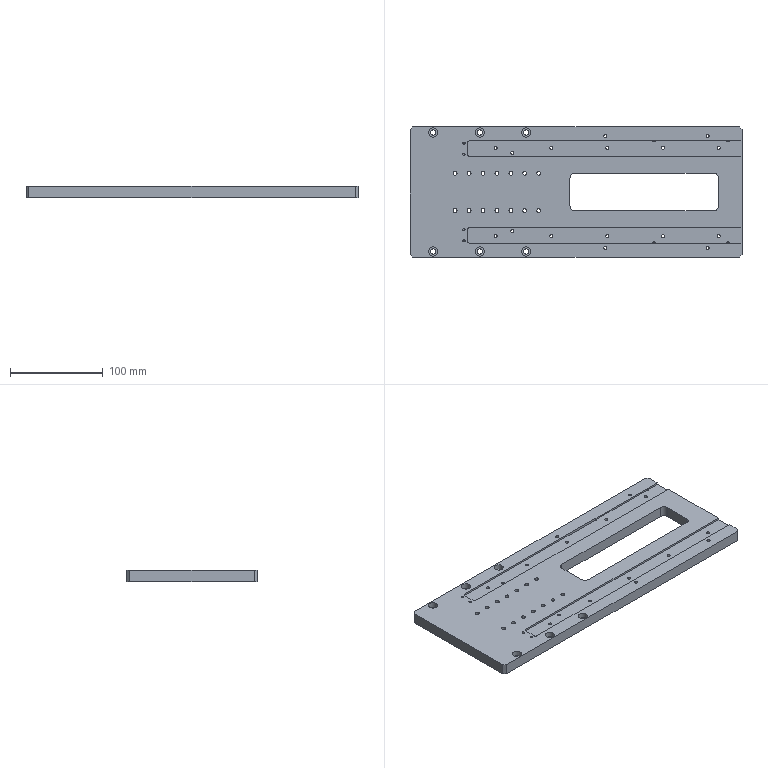NC program | NX | posted with a generic post | part box 357 x 140 x 12 mm
Lines 1 to 37 of 6551:
N10 G17 G21 G94 G90
(DRILLING_COPY_1 , TOOL : D6A45)
N12 T01 M6
N14 G54
N16 G17 G0 G90 X22.5 Y0. B0. C0. S9500 M3
N18 G43 Z30. H1
N20 G94 G81 G98 Z-1. F250. R3.
N22 X-60.
N24 X-22.5
N26 X59.5
N28 G80
N30 G0 X59.5 Y0. Z30.
N32 M5
(DRILLING_COPY_COPY_COPY_COPY_COPY , TOOL : 4.2ZT)
N34 T04 M6
N36 G54
N38 G17 G0 G90 X22.5 Y0. B0. C0. S2000 M3
N40 G43 Z30. H4
N42 G94 G83 G98 Z-13.762 F300. Q2. R3.
N44 X-22.5
N46 G80
N48 G0 X-22.5 Y0. Z30.
(DRILLING_COPY_COPY_COPY_COPY_COPY_COPY , TOOL : 4.2ZT)
N50 X-60.
N52 G83 Z-11.262 F300. Q2. R3.
N54 X59.5
N56 G80
N58 G0 X59.5 Y0. Z30.
N60 M5